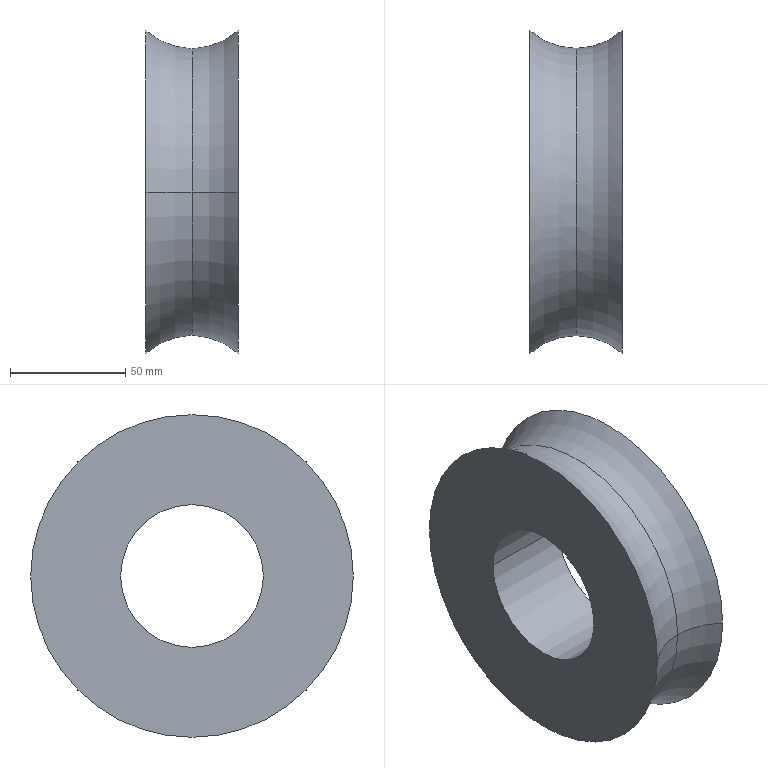Part | SolidWorks | features ICE 1, Revolution 1 | 1 solid | 8 faces | box 40 x 140 x 140 mm | volume 406899 mm3 | torus 4 | cylinder 2 | plane 2 | commonest cylinder face diameters 62 x2
STEP:
#1=CARTESIAN_POINT('',(-20.,-70.,0.));
#2=VERTEX_POINT('',#1);
#3=CARTESIAN_POINT('',(0.,-62.361,0.));
#4=VERTEX_POINT('',#3);
#5=CARTESIAN_POINT('',(0.,-92.361,0.));
#6=DIRECTION('',(0.,0.,-1.));
#7=DIRECTION('',(-1.,0.,0.));
#8=AXIS2_PLACEMENT_3D('',#5,#6,#7);
#9=CIRCLE('',#8,30.);
#10=EDGE_CURVE('',#2,#4,#9,.T.);
#11=ORIENTED_EDGE('',*,*,#10,.T.);
#12=CARTESIAN_POINT('',(0.,62.361,0.));
#13=VERTEX_POINT('',#12);
#14=CARTESIAN_POINT('',(0.,0.,0.));
#15=DIRECTION('',(-1.,0.,0.));
#16=DIRECTION('',(0.,-1.,0.));
#17=AXIS2_PLACEMENT_3D('',#14,#15,#16);
#18=CIRCLE('',#17,62.361);
#19=EDGE_CURVE('',#4,#13,#18,.T.);
#20=ORIENTED_EDGE('',*,*,#19,.T.);
#21=CARTESIAN_POINT('',(-20.,70.,0.));
#22=VERTEX_POINT('',#21);
#23=CARTESIAN_POINT('',(0.,92.361,0.));
#24=DIRECTION('',(0.,0.,1.));
#25=DIRECTION('',(0.,-1.,0.));
#26=AXIS2_PLACEMENT_3D('',#23,#24,#25);
#27=CIRCLE('',#26,30.);
#28=EDGE_CURVE('',#22,#13,#27,.T.);
#29=ORIENTED_EDGE('',*,*,#28,.F.);
#30=CARTESIAN_POINT('',(-20.,0.,0.));
#31=DIRECTION('',(-1.,0.,0.));
#32=DIRECTION('',(0.,-1.,0.));
#33=AXIS2_PLACEMENT_3D('',#30,#31,#32);
#34=CIRCLE('',#33,70.);
#35=EDGE_CURVE('',#2,#22,#34,.T.);
#36=ORIENTED_EDGE('',*,*,#35,.F.);
#37=EDGE_LOOP('',(#11,#20,#29,#36));
#38=FACE_OUTER_BOUND('',#37,.T.);
#39=CARTESIAN_POINT('',(0.,0.,0.));
#40=DIRECTION('',(-1.,0.,0.));
#41=DIRECTION('',(0.,-1.,0.));
#42=AXIS2_PLACEMENT_3D('',#39,#40,#41);
#43=TOROIDAL_SURFACE('',#42,92.361,30.);
#44=ADVANCED_FACE('',(#38),#43,.F.);
#45=ORIENTED_EDGE('',*,*,#28,.T.);
#46=CARTESIAN_POINT('',(0.,0.,0.));
#47=DIRECTION('',(-1.,0.,0.));
#48=DIRECTION('',(0.,-1.,0.));
#49=AXIS2_PLACEMENT_3D('',#46,#47,#48);
#50=CIRCLE('',#49,62.361);
#51=EDGE_CURVE('',#13,#4,#50,.T.);
#52=ORIENTED_EDGE('',*,*,#51,.T.);
#53=ORIENTED_EDGE('',*,*,#10,.F.);
#54=CARTESIAN_POINT('',(-20.,0.,0.));
#55=DIRECTION('',(-1.,0.,0.));
#56=DIRECTION('',(0.,-1.,0.));
#57=AXIS2_PLACEMENT_3D('',#54,#55,#56);
#58=CIRCLE('',#57,70.);
#59=EDGE_CURVE('',#22,#2,#58,.T.);
#60=ORIENTED_EDGE('',*,*,#59,.F.);
#61=EDGE_LOOP('',(#45,#52,#53,#60));
#62=FACE_OUTER_BOUND('',#61,.T.);
#63=CARTESIAN_POINT('',(0.,0.,0.));
#64=DIRECTION('',(-1.,0.,0.));
#65=DIRECTION('',(0.,-1.,0.));
#66=AXIS2_PLACEMENT_3D('',#63,#64,#65);
#67=TOROIDAL_SURFACE('',#66,92.361,30.);
#68=ADVANCED_FACE('',(#62),#67,.F.);
#69=CARTESIAN_POINT('',(-20.,-31.,0.));
#70=VERTEX_POINT('',#69);
#71=CARTESIAN_POINT('',(-20.,31.,0.));
#72=VERTEX_POINT('',#71);
#73=CARTESIAN_POINT('',(-20.,0.,0.));
#74=DIRECTION('',(1.,0.,0.));
#75=DIRECTION('',(0.,1.,0.));
#76=AXIS2_PLACEMENT_3D('',#73,#74,#75);
#77=CIRCLE('',#76,31.);
#78=EDGE_CURVE('',#70,#72,#77,.T.);
#79=ORIENTED_EDGE('',*,*,#78,.F.);
#80=CARTESIAN_POINT('',(20.,-31.,0.));
#81=VERTEX_POINT('',#80);
#82=CARTESIAN_POINT('',(-20.,-31.,0.));
#83=DIRECTION('',(1.,0.,0.));
#84=VECTOR('',#83,1000.);
#85=LINE('',#82,#84);
#86=EDGE_CURVE('',#70,#81,#85,.T.);
#87=ORIENTED_EDGE('',*,*,#86,.T.);
#88=CARTESIAN_POINT('',(20.,31.,0.));
#89=VERTEX_POINT('',#88);
#90=CARTESIAN_POINT('',(20.,0.,0.));
#91=DIRECTION('',(1.,0.,0.));
#92=DIRECTION('',(0.,1.,0.));
#93=AXIS2_PLACEMENT_3D('',#90,#91,#92);
#94=CIRCLE('',#93,31.);
#95=EDGE_CURVE('',#81,#89,#94,.T.);
#96=ORIENTED_EDGE('',*,*,#95,.T.);
#97=CARTESIAN_POINT('',(-20.,31.,0.));
#98=DIRECTION('',(1.,0.,0.));
#99=VECTOR('',#98,1000.);
#100=LINE('',#97,#99);
#101=EDGE_CURVE('',#72,#89,#100,.T.);
#102=ORIENTED_EDGE('',*,*,#101,.F.);
#103=EDGE_LOOP('',(#79,#87,#96,#102));
#104=FACE_OUTER_BOUND('',#103,.T.);
#105=CARTESIAN_POINT('',(-20.,0.,0.));
#106=DIRECTION('',(1.,0.,0.));
#107=DIRECTION('',(0.,1.,0.));
#108=AXIS2_PLACEMENT_3D('',#105,#106,#107);
#109=CYLINDRICAL_SURFACE('',#108,31.);
#110=ADVANCED_FACE('',(#104),#109,.F.);
#111=ORIENTED_EDGE('',*,*,#51,.F.);
#112=CARTESIAN_POINT('',(20.,70.,0.));
#113=VERTEX_POINT('',#112);
#114=CARTESIAN_POINT('',(0.,92.361,0.));
#115=DIRECTION('',(0.,0.,1.));
#116=DIRECTION('',(0.,-1.,0.));
#117=AXIS2_PLACEMENT_3D('',#114,#115,#116);
#118=CIRCLE('',#117,30.);
#119=EDGE_CURVE('',#13,#113,#118,.T.);
#120=ORIENTED_EDGE('',*,*,#119,.T.);
#121=CARTESIAN_POINT('',(20.,-70.,0.));
#122=VERTEX_POINT('',#121);
#123=CARTESIAN_POINT('',(20.,0.,0.));
#124=DIRECTION('',(-1.,0.,0.));
#125=DIRECTION('',(0.,-1.,0.));
#126=AXIS2_PLACEMENT_3D('',#123,#124,#125);
#127=CIRCLE('',#126,70.);
#128=EDGE_CURVE('',#113,#122,#127,.T.);
#129=ORIENTED_EDGE('',*,*,#128,.T.);
#130=CARTESIAN_POINT('',(0.,-92.361,0.));
#131=DIRECTION('',(0.,0.,-1.));
#132=DIRECTION('',(-1.,0.,0.));
#133=AXIS2_PLACEMENT_3D('',#130,#131,#132);
#134=CIRCLE('',#133,30.);
#135=EDGE_CURVE('',#4,#122,#134,.T.);
#136=ORIENTED_EDGE('',*,*,#135,.F.);
#137=EDGE_LOOP('',(#111,#120,#129,#136));
#138=FACE_OUTER_BOUND('',#137,.T.);
#139=CARTESIAN_POINT('',(0.,0.,0.));
#140=DIRECTION('',(-1.,0.,0.));
#141=DIRECTION('',(0.,-1.,0.));
#142=AXIS2_PLACEMENT_3D('',#139,#140,#141);
#143=TOROIDAL_SURFACE('',#142,92.361,30.);
#144=ADVANCED_FACE('',(#138),#143,.F.);
#145=ORIENTED_EDGE('',*,*,#19,.F.);
#146=ORIENTED_EDGE('',*,*,#135,.T.);
#147=CARTESIAN_POINT('',(20.,0.,0.));
#148=DIRECTION('',(-1.,0.,0.));
#149=DIRECTION('',(0.,-1.,0.));
#150=AXIS2_PLACEMENT_3D('',#147,#148,#149);
#151=CIRCLE('',#150,70.);
#152=EDGE_CURVE('',#122,#113,#151,.T.);
#153=ORIENTED_EDGE('',*,*,#152,.T.);
#154=ORIENTED_EDGE('',*,*,#119,.F.);
#155=EDGE_LOOP('',(#145,#146,#153,#154));
#156=FACE_OUTER_BOUND('',#155,.T.);
#157=CARTESIAN_POINT('',(0.,0.,0.));
#158=DIRECTION('',(-1.,0.,0.));
#159=DIRECTION('',(0.,-1.,0.));
#160=AXIS2_PLACEMENT_3D('',#157,#158,#159);
#161=TOROIDAL_SURFACE('',#160,92.361,30.);
#162=ADVANCED_FACE('',(#156),#161,.F.);
#163=CARTESIAN_POINT('',(-20.,0.,0.));
#164=DIRECTION('',(1.,0.,0.));
#165=DIRECTION('',(0.,1.,0.));
#166=AXIS2_PLACEMENT_3D('',#163,#164,#165);
#167=CIRCLE('',#166,31.);
#168=EDGE_CURVE('',#72,#70,#167,.T.);
#169=ORIENTED_EDGE('',*,*,#168,.T.);
#170=ORIENTED_EDGE('',*,*,#78,.T.);
#171=EDGE_LOOP('',(#169,#170));
#172=FACE_BOUND('',#171,.T.);
#173=ORIENTED_EDGE('',*,*,#35,.T.);
#174=ORIENTED_EDGE('',*,*,#59,.T.);
#175=EDGE_LOOP('',(#173,#174));
#176=FACE_OUTER_BOUND('',#175,.T.);
#177=CARTESIAN_POINT('',(-20.,70.,0.));
#178=DIRECTION('',(1.,0.,0.));
#179=DIRECTION('',(0.,1.,0.));
#180=AXIS2_PLACEMENT_3D('',#177,#178,#179);
#181=PLANE('',#180);
#182=ADVANCED_FACE('',(#172,#176),#181,.F.);
#183=CARTESIAN_POINT('',(20.,0.,0.));
#184=DIRECTION('',(1.,0.,0.));
#185=DIRECTION('',(0.,1.,0.));
#186=AXIS2_PLACEMENT_3D('',#183,#184,#185);
#187=CIRCLE('',#186,31.);
#188=EDGE_CURVE('',#89,#81,#187,.T.);
#189=ORIENTED_EDGE('',*,*,#188,.F.);
#190=ORIENTED_EDGE('',*,*,#95,.F.);
#191=EDGE_LOOP('',(#189,#190));
#192=FACE_BOUND('',#191,.T.);
#193=ORIENTED_EDGE('',*,*,#152,.F.);
#194=ORIENTED_EDGE('',*,*,#128,.F.);
#195=EDGE_LOOP('',(#193,#194));
#196=FACE_OUTER_BOUND('',#195,.T.);
#197=CARTESIAN_POINT('',(20.,70.,0.));
#198=DIRECTION('',(-1.,0.,0.));
#199=DIRECTION('',(0.,-1.,0.));
#200=AXIS2_PLACEMENT_3D('',#197,#198,#199);
#201=PLANE('',#200);
#202=ADVANCED_FACE('',(#192,#196),#201,.F.);
#203=ORIENTED_EDGE('',*,*,#86,.F.);
#204=ORIENTED_EDGE('',*,*,#168,.F.);
#205=ORIENTED_EDGE('',*,*,#101,.T.);
#206=ORIENTED_EDGE('',*,*,#188,.T.);
#207=EDGE_LOOP('',(#203,#204,#205,#206));
#208=FACE_OUTER_BOUND('',#207,.T.);
#209=CARTESIAN_POINT('',(-20.,0.,0.));
#210=DIRECTION('',(1.,0.,0.));
#211=DIRECTION('',(0.,1.,0.));
#212=AXIS2_PLACEMENT_3D('',#209,#210,#211);
#213=CYLINDRICAL_SURFACE('',#212,31.);
#214=ADVANCED_FACE('',(#208),#213,.F.);
#215=CLOSED_SHELL('',(#44,#68,#110,#144,#162,#182,#202,#214));
#216=MANIFOLD_SOLID_BREP('',#215);
#217=CARTESIAN_POINT('',(0.,0.,0.));
#218=DIRECTION('',(0.,0.,1.));
#219=DIRECTION('',(1.,0.,0.));
#220=AXIS2_PLACEMENT_3D('',#217,#218,#219);
#221=(LENGTH_UNIT()NAMED_UNIT(*)SI_UNIT(.MILLI.,.METRE.));
#222=UNCERTAINTY_MEASURE_WITH_UNIT(LENGTH_MEASURE(0.00001),#221,'','');
#223=(NAMED_UNIT(*)PLANE_ANGLE_UNIT()SI_UNIT($,.RADIAN.));
#224=(NAMED_UNIT(*)SI_UNIT($,.STERADIAN.)SOLID_ANGLE_UNIT());
#225=(GEOMETRIC_REPRESENTATION_CONTEXT(3)GLOBAL_UNCERTAINTY_ASSIGNED_CONTEXT((#222))GLOBAL_UNIT_ASSIGNED_CONTEXT((#221,#223,#224))REPRESENTATION_CONTEXT('',''));
#226=ADVANCED_BREP_SHAPE_REPRESENTATION('',(#216,#220),#225);